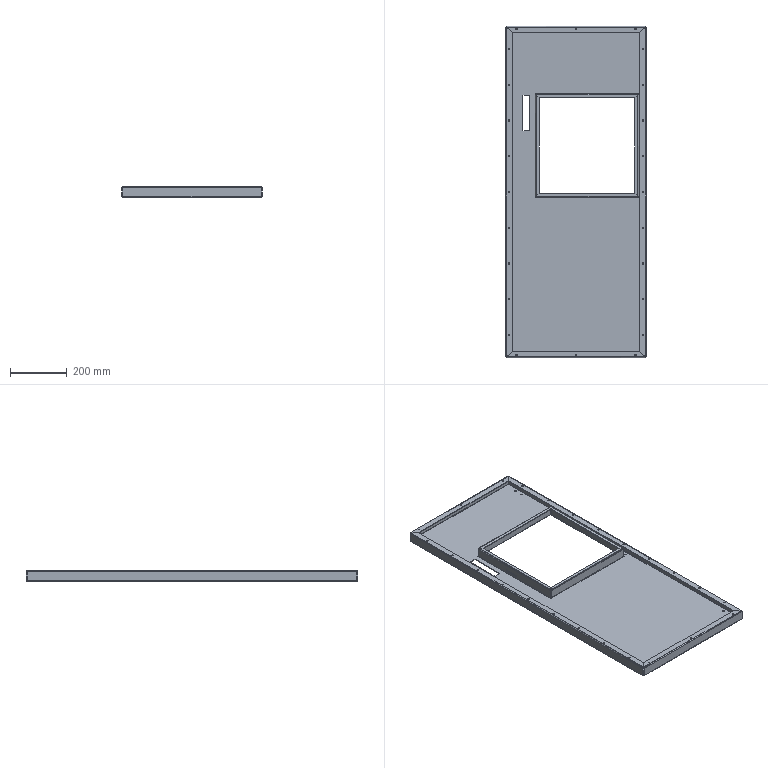Part | SolidWorks | 1 solid | 214 faces | box 494.5 x 1168 x 37 mm | volume 1696990 mm3 | cylinder 100 | plane 82 | spline 32 | commonest cylinder face diameters 5 x68 1.473 x16 6.473 x16